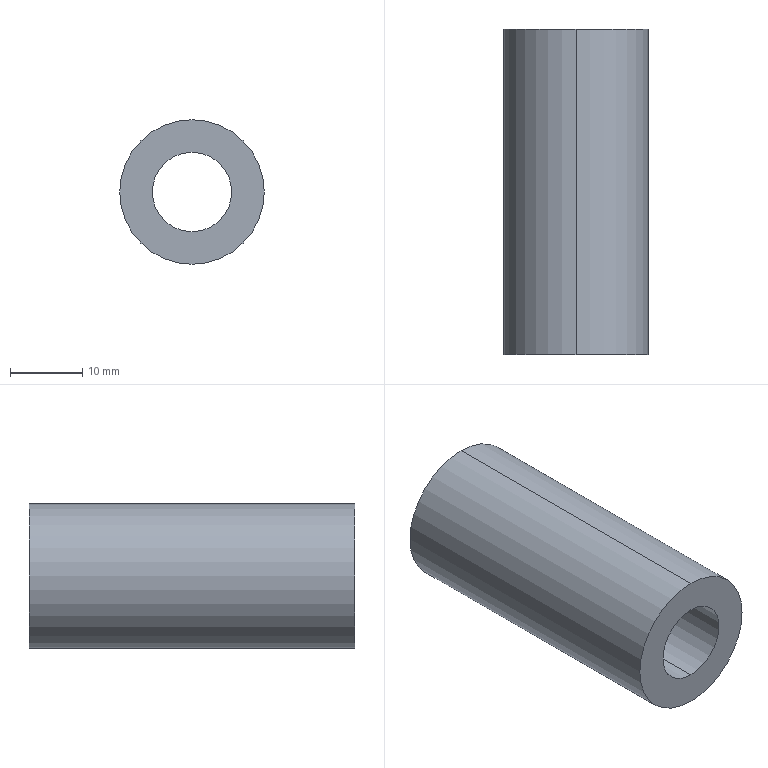Part | SolidWorks | features BaseBody 1 | 1 solid | 6 faces | box 20 x 45 x 20 mm | volume 9861 mm3 | cylinder 4 | plane 2 | commonest cylinder face diameters 11 x2 20 x2
STEP:
#1=CARTESIAN_POINT('',(0.,45.,-10.));
#2=VERTEX_POINT('',#1);
#3=CARTESIAN_POINT('',(0.,45.,10.));
#4=VERTEX_POINT('',#3);
#5=CARTESIAN_POINT('',(0.,45.,0.));
#6=DIRECTION('',(0.,-1.,0.));
#7=DIRECTION('',(0.,0.,-1.));
#8=AXIS2_PLACEMENT_3D('',#5,#6,#7);
#9=CIRCLE('',#8,10.);
#10=EDGE_CURVE('',#2,#4,#9,.T.);
#11=ORIENTED_EDGE('',*,*,#10,.T.);
#12=CARTESIAN_POINT('',(0.,0.,10.));
#13=VERTEX_POINT('',#12);
#14=CARTESIAN_POINT('',(0.,45.,10.));
#15=DIRECTION('',(0.,-1.,0.));
#16=VECTOR('',#15,1000.);
#17=LINE('',#14,#16);
#18=EDGE_CURVE('',#4,#13,#17,.T.);
#19=ORIENTED_EDGE('',*,*,#18,.T.);
#20=CARTESIAN_POINT('',(0.,0.,-10.));
#21=VERTEX_POINT('',#20);
#22=CARTESIAN_POINT('',(0.,0.,0.));
#23=DIRECTION('',(0.,1.,0.));
#24=DIRECTION('',(0.,0.,-1.));
#25=AXIS2_PLACEMENT_3D('',#22,#23,#24);
#26=CIRCLE('',#25,10.);
#27=EDGE_CURVE('',#13,#21,#26,.T.);
#28=ORIENTED_EDGE('',*,*,#27,.T.);
#29=CARTESIAN_POINT('',(0.,45.,-10.));
#30=DIRECTION('',(0.,-1.,0.));
#31=VECTOR('',#30,1000.);
#32=LINE('',#29,#31);
#33=EDGE_CURVE('',#2,#21,#32,.T.);
#34=ORIENTED_EDGE('',*,*,#33,.F.);
#35=EDGE_LOOP('',(#11,#19,#28,#34));
#36=FACE_OUTER_BOUND('',#35,.T.);
#37=CARTESIAN_POINT('',(0.,45.,0.));
#38=DIRECTION('',(0.,-1.,0.));
#39=DIRECTION('',(0.,0.,-1.));
#40=AXIS2_PLACEMENT_3D('',#37,#38,#39);
#41=CYLINDRICAL_SURFACE('',#40,10.);
#42=ADVANCED_FACE('',(#36),#41,.T.);
#43=CARTESIAN_POINT('',(0.,45.,5.5));
#44=VERTEX_POINT('',#43);
#45=CARTESIAN_POINT('',(0.,45.,-5.5));
#46=VERTEX_POINT('',#45);
#47=CARTESIAN_POINT('',(0.,45.,0.));
#48=DIRECTION('',(0.,-1.,0.));
#49=DIRECTION('',(0.,0.,-1.));
#50=AXIS2_PLACEMENT_3D('',#47,#48,#49);
#51=CIRCLE('',#50,5.5);
#52=EDGE_CURVE('',#44,#46,#51,.T.);
#53=ORIENTED_EDGE('',*,*,#52,.F.);
#54=CARTESIAN_POINT('',(0.,0.,5.5));
#55=VERTEX_POINT('',#54);
#56=CARTESIAN_POINT('',(0.,45.,5.5));
#57=DIRECTION('',(0.,-1.,0.));
#58=VECTOR('',#57,1000.);
#59=LINE('',#56,#58);
#60=EDGE_CURVE('',#44,#55,#59,.T.);
#61=ORIENTED_EDGE('',*,*,#60,.T.);
#62=CARTESIAN_POINT('',(0.,0.,-5.5));
#63=VERTEX_POINT('',#62);
#64=CARTESIAN_POINT('',(0.,0.,0.));
#65=DIRECTION('',(0.,-1.,0.));
#66=DIRECTION('',(0.,0.,-1.));
#67=AXIS2_PLACEMENT_3D('',#64,#65,#66);
#68=CIRCLE('',#67,5.5);
#69=EDGE_CURVE('',#55,#63,#68,.T.);
#70=ORIENTED_EDGE('',*,*,#69,.T.);
#71=CARTESIAN_POINT('',(0.,45.,-5.5));
#72=DIRECTION('',(0.,-1.,0.));
#73=VECTOR('',#72,1000.);
#74=LINE('',#71,#73);
#75=EDGE_CURVE('',#46,#63,#74,.T.);
#76=ORIENTED_EDGE('',*,*,#75,.F.);
#77=EDGE_LOOP('',(#53,#61,#70,#76));
#78=FACE_OUTER_BOUND('',#77,.T.);
#79=CARTESIAN_POINT('',(0.,45.,0.));
#80=DIRECTION('',(0.,-1.,0.));
#81=DIRECTION('',(0.,0.,-1.));
#82=AXIS2_PLACEMENT_3D('',#79,#80,#81);
#83=CYLINDRICAL_SURFACE('',#82,5.5);
#84=ADVANCED_FACE('',(#78),#83,.F.);
#85=ORIENTED_EDGE('',*,*,#18,.F.);
#86=CARTESIAN_POINT('',(0.,45.,0.));
#87=DIRECTION('',(0.,-1.,0.));
#88=DIRECTION('',(0.,0.,-1.));
#89=AXIS2_PLACEMENT_3D('',#86,#87,#88);
#90=CIRCLE('',#89,10.);
#91=EDGE_CURVE('',#4,#2,#90,.T.);
#92=ORIENTED_EDGE('',*,*,#91,.T.);
#93=ORIENTED_EDGE('',*,*,#33,.T.);
#94=CARTESIAN_POINT('',(0.,0.,0.));
#95=DIRECTION('',(0.,1.,0.));
#96=DIRECTION('',(0.,0.,-1.));
#97=AXIS2_PLACEMENT_3D('',#94,#95,#96);
#98=CIRCLE('',#97,10.);
#99=EDGE_CURVE('',#21,#13,#98,.T.);
#100=ORIENTED_EDGE('',*,*,#99,.T.);
#101=EDGE_LOOP('',(#85,#92,#93,#100));
#102=FACE_OUTER_BOUND('',#101,.T.);
#103=CARTESIAN_POINT('',(0.,45.,0.));
#104=DIRECTION('',(0.,-1.,0.));
#105=DIRECTION('',(0.,0.,-1.));
#106=AXIS2_PLACEMENT_3D('',#103,#104,#105);
#107=CYLINDRICAL_SURFACE('',#106,10.);
#108=ADVANCED_FACE('',(#102),#107,.T.);
#109=CARTESIAN_POINT('',(0.,0.,0.));
#110=DIRECTION('',(0.,-1.,0.));
#111=DIRECTION('',(0.,0.,-1.));
#112=AXIS2_PLACEMENT_3D('',#109,#110,#111);
#113=CIRCLE('',#112,5.5);
#114=EDGE_CURVE('',#63,#55,#113,.T.);
#115=ORIENTED_EDGE('',*,*,#114,.F.);
#116=ORIENTED_EDGE('',*,*,#69,.F.);
#117=EDGE_LOOP('',(#115,#116));
#118=FACE_BOUND('',#117,.T.);
#119=ORIENTED_EDGE('',*,*,#99,.F.);
#120=ORIENTED_EDGE('',*,*,#27,.F.);
#121=EDGE_LOOP('',(#119,#120));
#122=FACE_OUTER_BOUND('',#121,.T.);
#123=CARTESIAN_POINT('',(0.,0.,0.));
#124=DIRECTION('',(0.,1.,0.));
#125=DIRECTION('',(0.,0.,1.));
#126=AXIS2_PLACEMENT_3D('',#123,#124,#125);
#127=PLANE('',#126);
#128=ADVANCED_FACE('',(#118,#122),#127,.F.);
#129=CARTESIAN_POINT('',(0.,45.,0.));
#130=DIRECTION('',(0.,-1.,0.));
#131=DIRECTION('',(0.,0.,-1.));
#132=AXIS2_PLACEMENT_3D('',#129,#130,#131);
#133=CIRCLE('',#132,5.5);
#134=EDGE_CURVE('',#46,#44,#133,.T.);
#135=ORIENTED_EDGE('',*,*,#134,.T.);
#136=ORIENTED_EDGE('',*,*,#52,.T.);
#137=EDGE_LOOP('',(#135,#136));
#138=FACE_BOUND('',#137,.T.);
#139=ORIENTED_EDGE('',*,*,#10,.F.);
#140=ORIENTED_EDGE('',*,*,#91,.F.);
#141=EDGE_LOOP('',(#139,#140));
#142=FACE_OUTER_BOUND('',#141,.T.);
#143=CARTESIAN_POINT('',(0.,45.,0.));
#144=DIRECTION('',(0.,1.,0.));
#145=DIRECTION('',(0.,0.,1.));
#146=AXIS2_PLACEMENT_3D('',#143,#144,#145);
#147=PLANE('',#146);
#148=ADVANCED_FACE('',(#138,#142),#147,.T.);
#149=ORIENTED_EDGE('',*,*,#60,.F.);
#150=ORIENTED_EDGE('',*,*,#134,.F.);
#151=ORIENTED_EDGE('',*,*,#75,.T.);
#152=ORIENTED_EDGE('',*,*,#114,.T.);
#153=EDGE_LOOP('',(#149,#150,#151,#152));
#154=FACE_OUTER_BOUND('',#153,.T.);
#155=CARTESIAN_POINT('',(0.,45.,0.));
#156=DIRECTION('',(0.,-1.,0.));
#157=DIRECTION('',(0.,0.,-1.));
#158=AXIS2_PLACEMENT_3D('',#155,#156,#157);
#159=CYLINDRICAL_SURFACE('',#158,5.5);
#160=ADVANCED_FACE('',(#154),#159,.F.);
#161=CLOSED_SHELL('',(#42,#84,#108,#128,#148,#160));
#162=MANIFOLD_SOLID_BREP('',#161);
#163=CARTESIAN_POINT('',(0.,0.,0.));
#164=DIRECTION('',(0.,0.,1.));
#165=DIRECTION('',(1.,0.,0.));
#166=AXIS2_PLACEMENT_3D('',#163,#164,#165);
#167=(LENGTH_UNIT()NAMED_UNIT(*)SI_UNIT(.MILLI.,.METRE.));
#168=UNCERTAINTY_MEASURE_WITH_UNIT(LENGTH_MEASURE(0.00001),#167,'','');
#169=(NAMED_UNIT(*)PLANE_ANGLE_UNIT()SI_UNIT($,.RADIAN.));
#170=(NAMED_UNIT(*)SI_UNIT($,.STERADIAN.)SOLID_ANGLE_UNIT());
#171=(GEOMETRIC_REPRESENTATION_CONTEXT(3)GLOBAL_UNCERTAINTY_ASSIGNED_CONTEXT((#168))GLOBAL_UNIT_ASSIGNED_CONTEXT((#167,#169,#170))REPRESENTATION_CONTEXT('',''));
#172=ADVANCED_BREP_SHAPE_REPRESENTATION('',(#162,#166),#171);